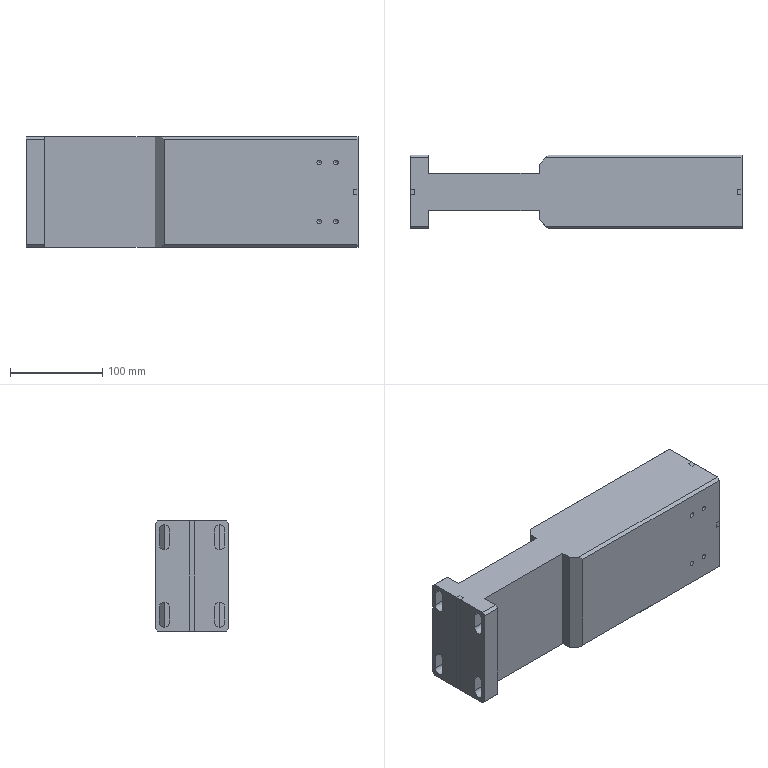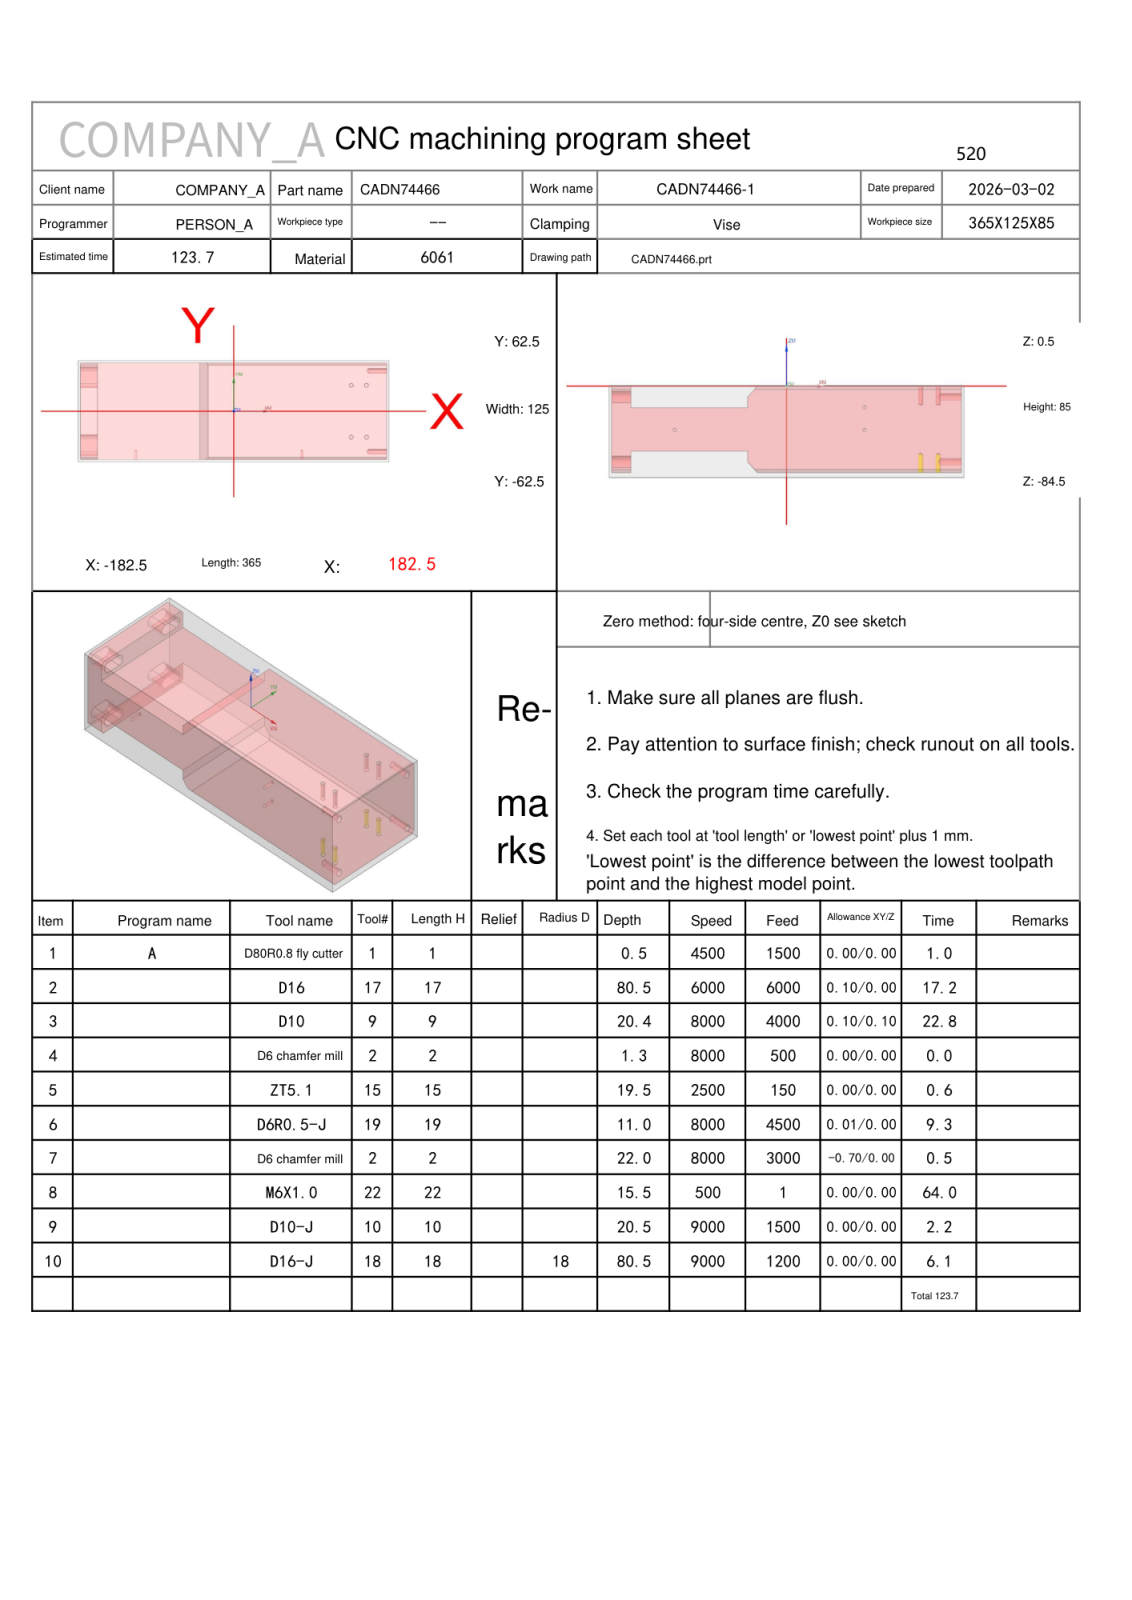NC program | NX | posted by the shop | part box 360 x 80 x 120 mm
Lines 1 to 871 of 7747:
%
O0001
(Machine time: 185.57 MIN)
(===Total Tool:9===)
(T1=D80R0.8 fly cutter D=80.  R=0.8  D-  H01 Z=0.    )
(T17=D16    D=16.  R=0.   D-  H17 Z=-80.  )
(T9=D10     D=10.  R=0.   D-  H09 Z=-19.9 )
(T2=D6 chamfer mill   D=6.   R=0.   D-  H02 Z=-21.5 )
(T15=ZT5.1  D=5.1  DR_a=118 D-  H15 Z=-19.  )
(T19=D6R0.5-J D=6.   R=0.5  D-  H19 Z=-10.5 )
(T22=M6X1.0 D=5.   DR_a=180 D-  H22 Z=-15.  )
(T10=D10-J  D=10.  R=0.   D10 H10 Z=-20.  )
(T18=D16-J  D=16.  R=0.   D18 H18 Z=-80.  )
G80 G90 G17 G49 G40
G91 G28 Z0
M01
N1 T01 M06
(D80R0.8 fly cutter  D=80. R=0.8 H=01 ce=0.00 di=0.00)
G00 G90 G54 X225. Y-50. M03 S4500
G43 H01 Z50.
M08
Z2.
G01 Z0.0 F1500.
X220.
X-220.
Y0.0
X220.
Y50.
X-220.
X-225.
Z2.
G00 Z50.
G91 G28 Z0.0
M05
M09
G91 G28 Z0.0
M01
N2 T17 M06
(D16  D=16. R=0. H=17 ce=0.10 di=0.00)
G00 G90 G54 X0.0 Y68.1 M03 S6000
G43 H17 Z50.
M08
Z.5
G01 X180. Z.358 F6000.
G02 X188.1 Y60. Z.348 I0.0 J-8.1
G01 Y-60. Z.253
G02 X180. Y-68.1 Z.243 I-8.1 J0.0
G01 X-180. Z-.04
G02 X-188.1 Y-60. Z-.05 I0.0 J8.1
G01 Y60. Z-.145
G02 X-180. Y68.1 Z-.155 I8.1 J0.0
G01 X180. Z-.439
G02 X188.1 Y60. Z-.449 I0.0 J-8.1
G01 Y-60. Z-.544
G02 X180. Y-68.1 Z-.554 I-8.1 J0.0
G01 X-180. Z-.837
G02 X-188.1 Y-60. Z-.847 I0.0 J8.1
G01 Y60. Z-.942
G02 X-180. Y68.1 Z-.952 I8.1 J0.0
G01 X180. Z-1.236
G02 X188.1 Y60. Z-1.246 I0.0 J-8.1
G01 Y-60. Z-1.341
G02 X180. Y-68.1 Z-1.351 I-8.1 J0.0
G01 X-180. Z-1.634
G02 X-188.1 Y-60. Z-1.645 I0.0 J8.1
G01 Y60. Z-1.739
G02 X-180. Y68.1 Z-1.749 I8.1 J0.0
G01 X180. Z-2.033
G02 X188.1 Y60. Z-2.043 I0.0 J-8.1
G01 Y-60. Z-2.138
G02 X180. Y-68.1 Z-2.148 I-8.1 J0.0
G01 X-180. Z-2.432
G02 X-188.1 Y-60. Z-2.442 I0.0 J8.1
G01 Y60. Z-2.536
G02 X-180. Y68.1 Z-2.546 I8.1 J0.0
G01 X180. Z-2.83
G02 X188.1 Y60. Z-2.84 I0.0 J-8.1
G01 Y-60. Z-2.935
G02 X180. Y-68.1 Z-2.945 I-8.1 J0.0
G01 X-180. Z-3.229
G02 X-188.1 Y-60. Z-3.239 I0.0 J8.1
G01 Y60. Z-3.333
G02 X-180. Y68.1 Z-3.343 I8.1 J0.0
G01 X180. Z-3.627
G02 X188.1 Y60. Z-3.637 I0.0 J-8.1
G01 Y-60. Z-3.732
G02 X180. Y-68.1 Z-3.742 I-8.1 J0.0
G01 X-180. Z-4.026
G02 X-188.1 Y-60. Z-4.036 I0.0 J8.1
G01 Y60. Z-4.13
G02 X-180. Y68.1 Z-4.14 I8.1 J0.0
G01 X180. Z-4.424
G02 X188.1 Y60. Z-4.434 I0.0 J-8.1
G01 Y-60. Z-4.529
G02 X180. Y-68.1 Z-4.539 I-8.1 J0.0
G01 X-180. Z-4.823
G02 X-188.1 Y-60. Z-4.833 I0.0 J8.1
G01 Y60. Z-4.927
G02 X-180. Y68.1 Z-4.937 I8.1 J0.0
G01 X180. Z-5.221
G02 X188.1 Y60. Z-5.231 I0.0 J-8.1
G01 Y-60. Z-5.326
G02 X180. Y-68.1 Z-5.336 I-8.1 J0.0
G01 X-180. Z-5.62
G02 X-188.1 Y-60. Z-5.63 I0.0 J8.1
G01 Y60. Z-5.724
G02 X-180. Y68.1 Z-5.734 I8.1 J0.0
G01 X180. Z-6.018
G02 X188.1 Y60. Z-6.028 I0.0 J-8.1
G01 Y-60. Z-6.123
G02 X180. Y-68.1 Z-6.133 I-8.1 J0.0
G01 X-180. Z-6.417
G02 X-188.1 Y-60. Z-6.427 I0.0 J8.1
G01 Y60. Z-6.521
G02 X-180. Y68.1 Z-6.531 I8.1 J0.0
G01 X180. Z-6.815
G02 X188.1 Y60. Z-6.825 I0.0 J-8.1
G01 Y-60. Z-6.92
G02 X180. Y-68.1 Z-6.93 I-8.1 J0.0
G01 X-180. Z-7.214
G02 X-188.1 Y-60. Z-7.224 I0.0 J8.1
G01 Y60. Z-7.318
G02 X-180. Y68.1 Z-7.328 I8.1 J0.0
G01 X180. Z-7.612
G02 X188.1 Y60. Z-7.622 I0.0 J-8.1
G01 Y-60. Z-7.717
G02 X180. Y-68.1 Z-7.727 I-8.1 J0.0
G01 X-180. Z-8.011
G02 X-188.1 Y-60. Z-8.021 I0.0 J8.1
G01 Y60. Z-8.115
G02 X-180. Y68.1 Z-8.125 I8.1 J0.0
G01 X180. Z-8.409
G02 X188.1 Y60. Z-8.419 I0.0 J-8.1
G01 Y-60. Z-8.514
G02 X180. Y-68.1 Z-8.524 I-8.1 J0.0
G01 X-180. Z-8.808
G02 X-188.1 Y-60. Z-8.818 I0.0 J8.1
G01 Y60. Z-8.912
G02 X-180. Y68.1 Z-8.922 I8.1 J0.0
G01 X180. Z-9.206
G02 X188.1 Y60. Z-9.216 I0.0 J-8.1
G01 Y-60. Z-9.311
G02 X180. Y-68.1 Z-9.321 I-8.1 J0.0
G01 X-180. Z-9.605
G02 X-188.1 Y-60. Z-9.615 I0.0 J8.1
G01 Y60. Z-9.709
G02 X-180. Y68.1 Z-9.719 I8.1 J0.0
G01 X180. Z-10.003
G02 X188.1 Y60. Z-10.013 I0.0 J-8.1
G01 Y-60. Z-10.108
G02 X180. Y-68.1 Z-10.118 I-8.1 J0.0
G01 X-180. Z-10.402
G02 X-188.1 Y-60. Z-10.412 I0.0 J8.1
G01 Y60. Z-10.506
G02 X-180. Y68.1 Z-10.516 I8.1 J0.0
G01 X180. Z-10.8
G02 X188.1 Y60. Z-10.81 I0.0 J-8.1
G01 Y-60. Z-10.905
G02 X180. Y-68.1 Z-10.915 I-8.1 J0.0
G01 X-180. Z-11.199
G02 X-188.1 Y-60. Z-11.209 I0.0 J8.1
G01 Y60. Z-11.303
G02 X-180. Y68.1 Z-11.314 I8.1 J0.0
G01 X180. Z-11.597
G02 X188.1 Y60. Z-11.607 I0.0 J-8.1
G01 Y-60. Z-11.702
G02 X180. Y-68.1 Z-11.712 I-8.1 J0.0
G01 X-180. Z-11.996
G02 X-188.1 Y-60. Z-12.006 I0.0 J8.1
G01 Y60. Z-12.101
G02 X-180. Y68.1 Z-12.111 I8.1 J0.0
G01 X180. Z-12.394
G02 X188.1 Y60. Z-12.404 I0.0 J-8.1
G01 Y-60. Z-12.499
G02 X180. Y-68.1 Z-12.509 I-8.1 J0.0
G01 X-180. Z-12.793
G02 X-188.1 Y-60. Z-12.803 I0.0 J8.1
G01 Y60. Z-12.898
G02 X-180. Y68.1 Z-12.908 I8.1 J0.0
G01 X180. Z-13.191
G02 X188.1 Y60. Z-13.201 I0.0 J-8.1
G01 Y-60. Z-13.296
G02 X180. Y-68.1 Z-13.306 I-8.1 J0.0
G01 X-180. Z-13.59
G02 X-188.1 Y-60. Z-13.6 I0.0 J8.1
G01 Y60. Z-13.695
G02 X-180. Y68.1 Z-13.705 I8.1 J0.0
G01 X180. Z-13.988
G02 X188.1 Y60. Z-13.998 I0.0 J-8.1
G01 Y-60. Z-14.093
G02 X180. Y-68.1 Z-14.103 I-8.1 J0.0
G01 X-180. Z-14.387
G02 X-188.1 Y-60. Z-14.397 I0.0 J8.1
G01 Y60. Z-14.492
G02 X-180. Y68.1 Z-14.502 I8.1 J0.0
G01 X180. Z-14.785
G02 X188.1 Y60. Z-14.796 I0.0 J-8.1
G01 Y-60. Z-14.89
G02 X180. Y-68.1 Z-14.9 I-8.1 J0.0
G01 X-180. Z-15.184
G02 X-188.1 Y-60. Z-15.194 I0.0 J8.1
G01 Y60. Z-15.289
G02 X-180. Y68.1 Z-15.299 I8.1 J0.0
G01 X180. Z-15.583
G02 X188.1 Y60. Z-15.593 I0.0 J-8.1
G01 Y-60. Z-15.687
G02 X180. Y-68.1 Z-15.697 I-8.1 J0.0
G01 X-180. Z-15.981
G02 X-188.1 Y-60. Z-15.991 I0.0 J8.1
G01 Y60. Z-16.086
G02 X-180. Y68.1 Z-16.096 I8.1 J0.0
G01 X180. Z-16.38
G02 X188.1 Y60. Z-16.39 I0.0 J-8.1
G01 Y-60. Z-16.484
G02 X180. Y-68.1 Z-16.494 I-8.1 J0.0
G01 X-180. Z-16.778
G02 X-188.1 Y-60. Z-16.788 I0.0 J8.1
G01 Y60. Z-16.883
G02 X-180. Y68.1 Z-16.893 I8.1 J0.0
G01 X180. Z-17.177
G02 X188.1 Y60. Z-17.187 I0.0 J-8.1
G01 Y-60. Z-17.281
G02 X180. Y-68.1 Z-17.291 I-8.1 J0.0
G01 X-180. Z-17.575
G02 X-188.1 Y-60. Z-17.585 I0.0 J8.1
G01 Y60. Z-17.68
G02 X-180. Y68.1 Z-17.69 I8.1 J0.0
G01 X180. Z-17.974
G02 X188.1 Y60. Z-17.984 I0.0 J-8.1
G01 Y-60. Z-18.078
G02 X180. Y-68.1 Z-18.088 I-8.1 J0.0
G01 X-180. Z-18.372
G02 X-188.1 Y-60. Z-18.382 I0.0 J8.1
G01 Y60. Z-18.477
G02 X-180. Y68.1 Z-18.487 I8.1 J0.0
G01 X180. Z-18.771
G02 X188.1 Y60. Z-18.781 I0.0 J-8.1
G01 Y-60. Z-18.875
G02 X180. Y-68.1 Z-18.885 I-8.1 J0.0
G01 X-180. Z-19.169
G02 X-188.1 Y-60. Z-19.179 I0.0 J8.1
G01 Y60. Z-19.274
G02 X-180. Y68.1 Z-19.284 I8.1 J0.0
G01 X180. Z-19.568
G02 X188.1 Y60. Z-19.578 I0.0 J-8.1
G01 Y-60. Z-19.672
G02 X180. Y-68.1 Z-19.682 I-8.1 J0.0
G01 X-180. Z-19.966
G02 X-188.1 Y-60. Z-19.976 I0.0 J8.1
G01 Y60. Z-20.071
G02 X-180. Y68.1 Z-20.081 I8.1 J0.0
G01 X180. Z-20.365
G02 X188.1 Y60. Z-20.375 I0.0 J-8.1
G01 Y-60. Z-20.469
G02 X180. Y-68.1 Z-20.479 I-8.1 J0.0
G01 X-180. Z-20.763
G02 X-188.1 Y-60. Z-20.773 I0.0 J8.1
G01 Y60. Z-20.868
G02 X-180. Y68.1 Z-20.878 I8.1 J0.0
G01 X180. Z-21.162
G02 X188.1 Y60. Z-21.172 I0.0 J-8.1
G01 Y-60. Z-21.266
G02 X180. Y-68.1 Z-21.276 I-8.1 J0.0
G01 X-180. Z-21.56
G02 X-188.1 Y-60. Z-21.57 I0.0 J8.1
G01 Y60. Z-21.665
G02 X-180. Y68.1 Z-21.675 I8.1 J0.0
G01 X180. Z-21.959
G02 X188.1 Y60. Z-21.969 I0.0 J-8.1
G01 Y-60. Z-22.063
G02 X180. Y-68.1 Z-22.073 I-8.1 J0.0
G01 X-180. Z-22.357
G02 X-188.1 Y-60. Z-22.367 I0.0 J8.1
G01 Y60. Z-22.462
G02 X-180. Y68.1 Z-22.472 I8.1 J0.0
G01 X180. Z-22.756
G02 X188.1 Y60. Z-22.766 I0.0 J-8.1
G01 Y-60. Z-22.86
G02 X180. Y-68.1 Z-22.87 I-8.1 J0.0
G01 X-180. Z-23.154
G02 X-188.1 Y-60. Z-23.164 I0.0 J8.1
G01 Y60. Z-23.259
G02 X-180. Y68.1 Z-23.269 I8.1 J0.0
G01 X180. Z-23.553
G02 X188.1 Y60. Z-23.563 I0.0 J-8.1
G01 Y-60. Z-23.657
G02 X180. Y-68.1 Z-23.667 I-8.1 J0.0
G01 X-180. Z-23.951
G02 X-188.1 Y-60. Z-23.961 I0.0 J8.1
G01 Y60. Z-24.056
G02 X-180. Y68.1 Z-24.066 I8.1 J0.0
G01 X180. Z-24.35
G02 X188.1 Y60. Z-24.36 I0.0 J-8.1
G01 Y-60. Z-24.454
G02 X180. Y-68.1 Z-24.465 I-8.1 J0.0
G01 X-180. Z-24.748
G02 X-188.1 Y-60. Z-24.758 I0.0 J8.1
G01 Y60. Z-24.853
G02 X-180. Y68.1 Z-24.863 I8.1 J0.0
G01 X180. Z-25.147
G02 X188.1 Y60. Z-25.157 I0.0 J-8.1
G01 Y-60. Z-25.252
G02 X180. Y-68.1 Z-25.262 I-8.1 J0.0
G01 X-180. Z-25.545
G02 X-188.1 Y-60. Z-25.555 I0.0 J8.1
G01 Y60. Z-25.65
G02 X-180. Y68.1 Z-25.66 I8.1 J0.0
G01 X180. Z-25.944
G02 X188.1 Y60. Z-25.954 I0.0 J-8.1
G01 Y-60. Z-26.049
G02 X180. Y-68.1 Z-26.059 I-8.1 J0.0
G01 X-180. Z-26.342
G02 X-188.1 Y-60. Z-26.352 I0.0 J8.1
G01 Y60. Z-26.447
G02 X-180. Y68.1 Z-26.457 I8.1 J0.0
G01 X180. Z-26.741
G02 X188.1 Y60. Z-26.751 I0.0 J-8.1
G01 Y-60. Z-26.846
G02 X180. Y-68.1 Z-26.856 I-8.1 J0.0
G01 X-180. Z-27.139
G02 X-188.1 Y-60. Z-27.149 I0.0 J8.1
G01 Y60. Z-27.244
G02 X-180. Y68.1 Z-27.254 I8.1 J0.0
G01 X180. Z-27.538
G02 X188.1 Y60. Z-27.548 I0.0 J-8.1
G01 Y-60. Z-27.643
G02 X180. Y-68.1 Z-27.653 I-8.1 J0.0
G01 X-180. Z-27.936
G02 X-188.1 Y-60. Z-27.947 I0.0 J8.1
G01 Y60. Z-28.041
G02 X-180. Y68.1 Z-28.051 I8.1 J0.0
G01 X180. Z-28.335
G02 X188.1 Y60. Z-28.345 I0.0 J-8.1
G01 Y-60. Z-28.44
G02 X180. Y-68.1 Z-28.45 I-8.1 J0.0
G01 X-180. Z-28.734
G02 X-188.1 Y-60. Z-28.744 I0.0 J8.1
G01 Y60. Z-28.838
G02 X-180. Y68.1 Z-28.848 I8.1 J0.0
G01 X180. Z-29.132
G02 X188.1 Y60. Z-29.142 I0.0 J-8.1
G01 Y-60. Z-29.237
G02 X180. Y-68.1 Z-29.247 I-8.1 J0.0
G01 X-180. Z-29.531
G02 X-188.1 Y-60. Z-29.541 I0.0 J8.1
G01 Y60. Z-29.635
G02 X-180. Y68.1 Z-29.645 I8.1 J0.0
G01 X180. Z-29.929
G02 X188.1 Y60. Z-29.939 I0.0 J-8.1
G01 Y-60. Z-30.034
G02 X180. Y-68.1 Z-30.044 I-8.1 J0.0
G01 X-180. Z-30.328
G02 X-188.1 Y-60. Z-30.338 I0.0 J8.1
G01 Y60. Z-30.432
G02 X-180. Y68.1 Z-30.442 I8.1 J0.0
G01 X180. Z-30.726
G02 X188.1 Y60. Z-30.736 I0.0 J-8.1
G01 Y-60. Z-30.831
G02 X180. Y-68.1 Z-30.841 I-8.1 J0.0
G01 X-180. Z-31.125
G02 X-188.1 Y-60. Z-31.135 I0.0 J8.1
G01 Y60. Z-31.229
G02 X-180. Y68.1 Z-31.239 I8.1 J0.0
G01 X180. Z-31.523
G02 X188.1 Y60. Z-31.533 I0.0 J-8.1
G01 Y-60. Z-31.628
G02 X180. Y-68.1 Z-31.638 I-8.1 J0.0
G01 X-180. Z-31.922
G02 X-188.1 Y-60. Z-31.932 I0.0 J8.1
G01 Y60. Z-32.026
G02 X-180. Y68.1 Z-32.036 I8.1 J0.0
G01 X180. Z-32.32
G02 X188.1 Y60. Z-32.33 I0.0 J-8.1
G01 Y-60. Z-32.425
G02 X180. Y-68.1 Z-32.435 I-8.1 J0.0
G01 X-180. Z-32.719
G02 X-188.1 Y-60. Z-32.729 I0.0 J8.1
G01 Y60. Z-32.823
G02 X-180. Y68.1 Z-32.833 I8.1 J0.0
G01 X180. Z-33.117
G02 X188.1 Y60. Z-33.127 I0.0 J-8.1
G01 Y-60. Z-33.222
G02 X180. Y-68.1 Z-33.232 I-8.1 J0.0
G01 X-180. Z-33.516
G02 X-188.1 Y-60. Z-33.526 I0.0 J8.1
G01 Y60. Z-33.62
G02 X-180. Y68.1 Z-33.63 I8.1 J0.0
G01 X180. Z-33.914
G02 X188.1 Y60. Z-33.924 I0.0 J-8.1
G01 Y-60. Z-34.019
G02 X180. Y-68.1 Z-34.029 I-8.1 J0.0
G01 X-180. Z-34.313
G02 X-188.1 Y-60. Z-34.323 I0.0 J8.1
G01 Y60. Z-34.417
G02 X-180. Y68.1 Z-34.427 I8.1 J0.0
G01 X180. Z-34.711
G02 X188.1 Y60. Z-34.721 I0.0 J-8.1
G01 Y-60. Z-34.816
G02 X180. Y-68.1 Z-34.826 I-8.1 J0.0
G01 X-180. Z-35.11
G02 X-188.1 Y-60. Z-35.12 I0.0 J8.1
G01 Y60. Z-35.214
G02 X-180. Y68.1 Z-35.224 I8.1 J0.0
G01 X180. Z-35.508
G02 X188.1 Y60. Z-35.518 I0.0 J-8.1
G01 Y-60. Z-35.613
G02 X180. Y-68.1 Z-35.623 I-8.1 J0.0
G01 X-180. Z-35.907
G02 X-188.1 Y-60. Z-35.917 I0.0 J8.1
G01 Y60. Z-36.011
G02 X-180. Y68.1 Z-36.021 I8.1 J0.0
G01 X180. Z-36.305
G02 X188.1 Y60. Z-36.315 I0.0 J-8.1
G01 Y-60. Z-36.41
G02 X180. Y-68.1 Z-36.42 I-8.1 J0.0
G01 X-180. Z-36.704
G02 X-188.1 Y-60. Z-36.714 I0.0 J8.1
G01 Y60. Z-36.808
G02 X-180. Y68.1 Z-36.818 I8.1 J0.0
G01 X180. Z-37.102
G02 X188.1 Y60. Z-37.112 I0.0 J-8.1
G01 Y-60. Z-37.207
G02 X180. Y-68.1 Z-37.217 I-8.1 J0.0
G01 X-180. Z-37.501
G02 X-188.1 Y-60. Z-37.511 I0.0 J8.1
G01 Y60. Z-37.605
G02 X-180. Y68.1 Z-37.616 I8.1 J0.0
G01 X180. Z-37.899
G02 X188.1 Y60. Z-37.909 I0.0 J-8.1
G01 Y-60. Z-38.004
G02 X180. Y-68.1 Z-38.014 I-8.1 J0.0
G01 X-180. Z-38.298
G02 X-188.1 Y-60. Z-38.308 I0.0 J8.1
G01 Y60. Z-38.403
G02 X-180. Y68.1 Z-38.413 I8.1 J0.0
G01 X180. Z-38.696
G02 X188.1 Y60. Z-38.706 I0.0 J-8.1
G01 Y-60. Z-38.801
G02 X180. Y-68.1 Z-38.811 I-8.1 J0.0
G01 X-180. Z-39.095
G02 X-188.1 Y-60. Z-39.105 I0.0 J8.1
G01 Y60. Z-39.2
G02 X-180. Y68.1 Z-39.21 I8.1 J0.0
G01 X180. Z-39.493
G02 X188.1 Y60. Z-39.503 I0.0 J-8.1
G01 Y-60. Z-39.598
G02 X180. Y-68.1 Z-39.608 I-8.1 J0.0
G01 X-180. Z-39.892
G02 X-188.1 Y-60. Z-39.902 I0.0 J8.1
G01 Y60. Z-39.997
G02 X-180. Y68.1 Z-40.007 I8.1 J0.0
G01 X180. Z-40.29
G02 X188.1 Y60. Z-40.3 I0.0 J-8.1
G01 Y-60. Z-40.395
G02 X180. Y-68.1 Z-40.405 I-8.1 J0.0
G01 X-180. Z-40.689
G02 X-188.1 Y-60. Z-40.699 I0.0 J8.1
G01 Y60. Z-40.794
G02 X-180. Y68.1 Z-40.804 I8.1 J0.0
G01 X180. Z-41.087
G02 X188.1 Y60. Z-41.097 I0.0 J-8.1
G01 Y-60. Z-41.192
G02 X180. Y-68.1 Z-41.202 I-8.1 J0.0
G01 X-180. Z-41.486
G02 X-188.1 Y-60. Z-41.496 I0.0 J8.1
G01 Y60. Z-41.591
G02 X-180. Y68.1 Z-41.601 I8.1 J0.0
G01 X180. Z-41.884
G02 X188.1 Y60. Z-41.895 I0.0 J-8.1
G01 Y-60. Z-41.989
G02 X180. Y-68.1 Z-41.999 I-8.1 J0.0
G01 X-180. Z-42.283
G02 X-188.1 Y-60. Z-42.293 I0.0 J8.1
G01 Y60. Z-42.388
G02 X-180. Y68.1 Z-42.398 I8.1 J0.0
G01 X180. Z-42.682
G02 X188.1 Y60. Z-42.692 I0.0 J-8.1
G01 Y-60. Z-42.786
G02 X180. Y-68.1 Z-42.796 I-8.1 J0.0
G01 X-180. Z-43.08
G02 X-188.1 Y-60. Z-43.09 I0.0 J8.1
G01 Y60. Z-43.185
G02 X-180. Y68.1 Z-43.195 I8.1 J0.0
G01 X180. Z-43.479
G02 X188.1 Y60. Z-43.489 I0.0 J-8.1
G01 Y-60. Z-43.583
G02 X180. Y-68.1 Z-43.593 I-8.1 J0.0
G01 X-180. Z-43.877
G02 X-188.1 Y-60. Z-43.887 I0.0 J8.1
G01 Y60. Z-43.982
G02 X-180. Y68.1 Z-43.992 I8.1 J0.0
G01 X180. Z-44.276
G02 X188.1 Y60. Z-44.286 I0.0 J-8.1
G01 Y-60. Z-44.38
G02 X180. Y-68.1 Z-44.39 I-8.1 J0.0
G01 X-180. Z-44.674
G02 X-188.1 Y-60. Z-44.684 I0.0 J8.1
G01 Y60. Z-44.779
G02 X-180. Y68.1 Z-44.789 I8.1 J0.0
G01 X180. Z-45.073
G02 X188.1 Y60. Z-45.083 I0.0 J-8.1
G01 Y-60. Z-45.177
G02 X180. Y-68.1 Z-45.187 I-8.1 J0.0
G01 X-180. Z-45.471
G02 X-188.1 Y-60. Z-45.481 I0.0 J8.1
G01 Y60. Z-45.576
G02 X-180. Y68.1 Z-45.586 I8.1 J0.0
G01 X180. Z-45.87
G02 X188.1 Y60. Z-45.88 I0.0 J-8.1
G01 Y-60. Z-45.974
G02 X180. Y-68.1 Z-45.984 I-8.1 J0.0
G01 X-180. Z-46.268
G02 X-188.1 Y-60. Z-46.278 I0.0 J8.1
G01 Y60. Z-46.373
G02 X-180. Y68.1 Z-46.383 I8.1 J0.0
G01 X180. Z-46.667
G02 X188.1 Y60. Z-46.677 I0.0 J-8.1
G01 Y-60. Z-46.771
G02 X180. Y-68.1 Z-46.781 I-8.1 J0.0
G01 X-180. Z-47.065
G02 X-188.1 Y-60. Z-47.075 I0.0 J8.1
G01 Y60. Z-47.17
G02 X-180. Y68.1 Z-47.18 I8.1 J0.0
G01 X180. Z-47.464
G02 X188.1 Y60. Z-47.474 I0.0 J-8.1
G01 Y-60. Z-47.568
G02 X180. Y-68.1 Z-47.578 I-8.1 J0.0
G01 X-180. Z-47.862
G02 X-188.1 Y-60. Z-47.872 I0.0 J8.1
G01 Y60. Z-47.967
G02 X-180. Y68.1 Z-47.977 I8.1 J0.0
G01 X180. Z-48.261
G02 X188.1 Y60. Z-48.271 I0.0 J-8.1
G01 Y-60. Z-48.365
G02 X180. Y-68.1 Z-48.375 I-8.1 J0.0
G01 X-180. Z-48.659
G02 X-188.1 Y-60. Z-48.669 I0.0 J8.1
G01 Y60. Z-48.764
G02 X-180. Y68.1 Z-48.774 I8.1 J0.0
G01 X180. Z-49.058
G02 X188.1 Y60. Z-49.068 I0.0 J-8.1
G01 Y-60. Z-49.162
G02 X180. Y-68.1 Z-49.172 I-8.1 J0.0
G01 X-180. Z-49.456
G02 X-188.1 Y-60. Z-49.466 I0.0 J8.1
G01 Y60. Z-49.561
G02 X-180. Y68.1 Z-49.571 I8.1 J0.0
G01 X180. Z-49.855
G02 X188.1 Y60. Z-49.865 I0.0 J-8.1
G01 Y-60. Z-49.959
G02 X180. Y-68.1 Z-49.969 I-8.1 J0.0
G01 X-180. Z-50.253
G02 X-188.1 Y-60. Z-50.263 I0.0 J8.1
G01 Y60. Z-50.358
G02 X-180. Y68.1 Z-50.368 I8.1 J0.0
G01 X180. Z-50.652
G02 X188.1 Y60. Z-50.662 I0.0 J-8.1
G01 Y-60. Z-50.756
G02 X180. Y-68.1 Z-50.766 I-8.1 J0.0
G01 X-180. Z-51.05
G02 X-188.1 Y-60. Z-51.06 I0.0 J8.1
G01 Y60. Z-51.155
G02 X-180. Y68.1 Z-51.165 I8.1 J0.0
G01 X180. Z-51.449
G02 X188.1 Y60. Z-51.459 I0.0 J-8.1
G01 Y-60. Z-51.553
G02 X180. Y-68.1 Z-51.564 I-8.1 J0.0
G01 X-180. Z-51.847
G02 X-188.1 Y-60. Z-51.857 I0.0 J8.1
G01 Y60. Z-51.952
G02 X-180. Y68.1 Z-51.962 I8.1 J0.0
G01 X180. Z-52.246
G02 X188.1 Y60. Z-52.256 I0.0 J-8.1
G01 Y-60. Z-52.351
G02 X180. Y-68.1 Z-52.361 I-8.1 J0.0
G01 X-180. Z-52.644
G02 X-188.1 Y-60. Z-52.654 I0.0 J8.1
G01 Y60. Z-52.749
G02 X-180. Y68.1 Z-52.759 I8.1 J0.0
G01 X180. Z-53.043
G02 X188.1 Y60. Z-53.053 I0.0 J-8.1
G01 Y-60. Z-53.148
G02 X180. Y-68.1 Z-53.158 I-8.1 J0.0
G01 X-180. Z-53.441
G02 X-188.1 Y-60. Z-53.451 I0.0 J8.1
G01 Y60. Z-53.546
G02 X-180. Y68.1 Z-53.556 I8.1 J0.0
G01 X180. Z-53.84
G02 X188.1 Y60. Z-53.85 I0.0 J-8.1
G01 Y-60. Z-53.945
G02 X180. Y-68.1 Z-53.955 I-8.1 J0.0
G01 X-180. Z-54.238
G02 X-188.1 Y-60. Z-54.248 I0.0 J8.1
G01 Y60. Z-54.343
G02 X-180. Y68.1 Z-54.353 I8.1 J0.0
G01 X180. Z-54.637
G02 X188.1 Y60. Z-54.647 I0.0 J-8.1
G01 Y-60. Z-54.742
G02 X180. Y-68.1 Z-54.752 I-8.1 J0.0
G01 X-180. Z-55.035
G02 X-188.1 Y-60. Z-55.046 I0.0 J8.1
G01 Y60. Z-55.14
G02 X-180. Y68.1 Z-55.15 I8.1 J0.0
G01 X180. Z-55.434
G02 X188.1 Y60. Z-55.444 I0.0 J-8.1
G01 Y-60. Z-55.539
G02 X180. Y-68.1 Z-55.549 I-8.1 J0.0
G01 X-180. Z-55.833
G02 X-188.1 Y-60. Z-55.843 I0.0 J8.1
G01 Y60. Z-55.937
G02 X-180. Y68.1 Z-55.947 I8.1 J0.0
G01 X180. Z-56.231
G02 X188.1 Y60. Z-56.241 I0.0 J-8.1
G01 Y-60. Z-56.336
G02 X180. Y-68.1 Z-56.346 I-8.1 J0.0
G01 X-180. Z-56.63
G02 X-188.1 Y-60. Z-56.64 I0.0 J8.1
G01 Y60. Z-56.734
G02 X-180. Y68.1 Z-56.744 I8.1 J0.0
G01 X180. Z-57.028
G02 X188.1 Y60. Z-57.038 I0.0 J-8.1
G01 Y-60. Z-57.133
G02 X180. Y-68.1 Z-57.143 I-8.1 J0.0
G01 X-180. Z-57.427
G02 X-188.1 Y-60. Z-57.437 I0.0 J8.1
G01 Y60. Z-57.531
G02 X-180. Y68.1 Z-57.541 I8.1 J0.0
G01 X180. Z-57.825
G02 X188.1 Y60. Z-57.835 I0.0 J-8.1
G01 Y-60. Z-57.93
G02 X180. Y-68.1 Z-57.94 I-8.1 J0.0
G01 X-180. Z-58.224
G02 X-188.1 Y-60. Z-58.234 I0.0 J8.1
G01 Y60. Z-58.328
G02 X-180. Y68.1 Z-58.338 I8.1 J0.0
G01 X180. Z-58.622
G02 X188.1 Y60. Z-58.632 I0.0 J-8.1
G01 Y-60. Z-58.727
G02 X180. Y-68.1 Z-58.737 I-8.1 J0.0
G01 X-180. Z-59.021
G02 X-188.1 Y-60. Z-59.031 I0.0 J8.1
G01 Y60. Z-59.125
G02 X-180. Y68.1 Z-59.135 I8.1 J0.0
G01 X180. Z-59.419
G02 X188.1 Y60. Z-59.429 I0.0 J-8.1
G01 Y-60. Z-59.524
G02 X180. Y-68.1 Z-59.534 I-8.1 J0.0
G01 X-180. Z-59.818
G02 X-188.1 Y-60. Z-59.828 I0.0 J8.1
G01 Y60. Z-59.922
G02 X-180. Y68.1 Z-59.932 I8.1 J0.0
G01 X180. Z-60.216
G02 X188.1 Y60. Z-60.226 I0.0 J-8.1
G01 Y-60. Z-60.321
G02 X180. Y-68.1 Z-60.331 I-8.1 J0.0
G01 X-180. Z-60.615
G02 X-188.1 Y-60. Z-60.625 I0.0 J8.1
G01 Y60. Z-60.719
G02 X-180. Y68.1 Z-60.729 I8.1 J0.0
G01 X180. Z-61.013
G02 X188.1 Y60. Z-61.023 I0.0 J-8.1
G01 Y-60. Z-61.118
G02 X180. Y-68.1 Z-61.128 I-8.1 J0.0
G01 X-180. Z-61.412
G02 X-188.1 Y-60. Z-61.422 I0.0 J8.1
G01 Y60. Z-61.516
G02 X-180. Y68.1 Z-61.526 I8.1 J0.0
G01 X180. Z-61.81
G02 X188.1 Y60. Z-61.82 I0.0 J-8.1
G01 Y-60. Z-61.915
G02 X180. Y-68.1 Z-61.925 I-8.1 J0.0
G01 X-180. Z-62.209
G02 X-188.1 Y-60. Z-62.219 I0.0 J8.1
G01 Y60. Z-62.313
G02 X-180. Y68.1 Z-62.323 I8.1 J0.0
G01 X180. Z-62.607
G02 X188.1 Y60. Z-62.617 I0.0 J-8.1
G01 Y-60. Z-62.712
G02 X180. Y-68.1 Z-62.722 I-8.1 J0.0
G01 X-180. Z-63.006
G02 X-188.1 Y-60. Z-63.016 I0.0 J8.1
G01 Y60. Z-63.11
G02 X-180. Y68.1 Z-63.12 I8.1 J0.0
G01 X180. Z-63.404
G02 X188.1 Y60. Z-63.414 I0.0 J-8.1
G01 Y-60. Z-63.509
G02 X180. Y-68.1 Z-63.519 I-8.1 J0.0
G01 X-180. Z-63.803
G02 X-188.1 Y-60. Z-63.813 I0.0 J8.1
G01 Y60. Z-63.907
G02 X-180. Y68.1 Z-63.917 I8.1 J0.0
G01 X180. Z-64.201
G02 X188.1 Y60. Z-64.211 I0.0 J-8.1
G01 Y-60. Z-64.306
G02 X180. Y-68.1 Z-64.316 I-8.1 J0.0
G01 X-180. Z-64.6
G02 X-188.1 Y-60. Z-64.61 I0.0 J8.1
G01 Y60. Z-64.704
G02 X-180. Y68.1 Z-64.715 I8.1 J0.0
G01 X180. Z-64.998
G02 X188.1 Y60. Z-65.008 I0.0 J-8.1
G01 Y-60. Z-65.103
G02 X180. Y-68.1 Z-65.113 I-8.1 J0.0
G01 X-180. Z-65.397
G02 X-188.1 Y-60. Z-65.407 I0.0 J8.1
G01 Y60. Z-65.502
G02 X-180. Y68.1 Z-65.512 I8.1 J0.0
G01 X180. Z-65.795
G02 X188.1 Y60. Z-65.805 I0.0 J-8.1
G01 Y-60. Z-65.9
G02 X180. Y-68.1 Z-65.91 I-8.1 J0.0
G01 X-180. Z-66.194
G02 X-188.1 Y-60. Z-66.204 I0.0 J8.1
G01 Y60. Z-66.299
G02 X-180. Y68.1 Z-66.309 I8.1 J0.0
G01 X180. Z-66.592
G02 X188.1 Y60. Z-66.602 I0.0 J-8.1
G01 Y-60. Z-66.697
G02 X180. Y-68.1 Z-66.707 I-8.1 J0.0
G01 X-180. Z-66.991
G02 X-188.1 Y-60. Z-67.001 I0.0 J8.1
G01 Y60. Z-67.096
G02 X-180. Y68.1 Z-67.106 I8.1 J0.0
G01 X180. Z-67.389
G02 X188.1 Y60. Z-67.399 I0.0 J-8.1
G01 Y-60. Z-67.494
G02 X180. Y-68.1 Z-67.504 I-8.1 J0.0
G01 X-180. Z-67.788
G02 X-188.1 Y-60. Z-67.798 I0.0 J8.1
G01 Y60. Z-67.893
G02 X-180. Y68.1 Z-67.903 I8.1 J0.0
G01 X180. Z-68.186
G02 X188.1 Y60. Z-68.197 I0.0 J-8.1
G01 Y-60. Z-68.291
G02 X180. Y-68.1 Z-68.301 I-8.1 J0.0
G01 X-180. Z-68.585
G02 X-188.1 Y-60. Z-68.595 I0.0 J8.1
G01 Y60. Z-68.69
G02 X-180. Y68.1 Z-68.7 I8.1 J0.0
G01 X180. Z-68.984
G02 X188.1 Y60. Z-68.994 I0.0 J-8.1
G01 Y-60. Z-69.088
G02 X180. Y-68.1 Z-69.098 I-8.1 J0.0
G01 X-180. Z-69.382
G02 X-188.1 Y-60. Z-69.392 I0.0 J8.1
G01 Y60. Z-69.487
G02 X-180. Y68.1 Z-69.497 I8.1 J0.0
G01 X180. Z-69.781
G02 X188.1 Y60. Z-69.791 I0.0 J-8.1
G01 Y-60. Z-69.885
G02 X180. Y-68.1 Z-69.895 I-8.1 J0.0
G01 X-180. Z-70.179
G02 X-188.1 Y-60. Z-70.189 I0.0 J8.1
G01 Y60. Z-70.284
G02 X-180. Y68.1 Z-70.294 I8.1 J0.0
G01 X180. Z-70.578
G02 X188.1 Y60. Z-70.588 I0.0 J-8.1
G01 Y-60. Z-70.682
G02 X180. Y-68.1 Z-70.692 I-8.1 J0.0
G01 X-180. Z-70.976
G02 X-188.1 Y-60. Z-70.986 I0.0 J8.1
G01 Y60. Z-71.081
G02 X-180. Y68.1 Z-71.091 I8.1 J0.0
G01 X180. Z-71.375
G02 X188.1 Y60. Z-71.385 I0.0 J-8.1
G01 Y-60. Z-71.479
G02 X180. Y-68.1 Z-71.489 I-8.1 J0.0
G01 X-180. Z-71.773
G02 X-188.1 Y-60. Z-71.783 I0.0 J8.1
G01 Y60. Z-71.878
G02 X-180. Y68.1 Z-71.888 I8.1 J0.0
G01 X180. Z-72.172
G02 X188.1 Y60. Z-72.182 I0.0 J-8.1
G01 Y-60. Z-72.276
G02 X180. Y-68.1 Z-72.286 I-8.1 J0.0
G01 X-180. Z-72.57
G02 X-188.1 Y-60. Z-72.58 I0.0 J8.1
G01 Y60. Z-72.675
G02 X-180. Y68.1 Z-72.685 I8.1 J0.0
G01 X180. Z-72.969
G02 X188.1 Y60. Z-72.979 I0.0 J-8.1
G01 Y-60. Z-73.073
G02 X180. Y-68.1 Z-73.083 I-8.1 J0.0
G01 X-180. Z-73.367
G02 X-188.1 Y-60. Z-73.377 I0.0 J8.1
G01 Y60. Z-73.472
G02 X-180. Y68.1 Z-73.482 I8.1 J0.0
G01 X180. Z-73.766
G02 X188.1 Y60. Z-73.776 I0.0 J-8.1
G01 Y-60. Z-73.87
G02 X180. Y-68.1 Z-73.88 I-8.1 J0.0
G01 X-180. Z-74.164
G02 X-188.1 Y-60. Z-74.174 I0.0 J8.1
G01 Y60. Z-74.269
G02 X-180. Y68.1 Z-74.279 I8.1 J0.0
G01 X180. Z-74.563
G02 X188.1 Y60. Z-74.573 I0.0 J-8.1
G01 Y-60. Z-74.667
G02 X180. Y-68.1 Z-74.677 I-8.1 J0.0
G01 X-180. Z-74.961
G02 X-188.1 Y-60. Z-74.971 I0.0 J8.1
G01 Y60. Z-75.066
G02 X-180. Y68.1 Z-75.076 I8.1 J0.0
G01 X180. Z-75.36
G02 X188.1 Y60. Z-75.37 I0.0 J-8.1
G01 Y-60. Z-75.464
G02 X180. Y-68.1 Z-75.474 I-8.1 J0.0
G01 X-180. Z-75.758
G02 X-188.1 Y-60. Z-75.768 I0.0 J8.1
G01 Y60. Z-75.863
G02 X-180. Y68.1 Z-75.873 I8.1 J0.0
G01 X180. Z-76.157
G02 X188.1 Y60. Z-76.167 I0.0 J-8.1
G01 Y-60. Z-76.261
G02 X180. Y-68.1 Z-76.271 I-8.1 J0.0
G01 X-180. Z-76.555
G02 X-188.1 Y-60. Z-76.565 I0.0 J8.1
G01 Y60. Z-76.66
G02 X-180. Y68.1 Z-76.67 I8.1 J0.0
G01 X180. Z-76.954
G02 X188.1 Y60. Z-76.964 I0.0 J-8.1
G01 Y-60. Z-77.058
G02 X180. Y-68.1 Z-77.068 I-8.1 J0.0
G01 X-180. Z-77.352
G02 X-188.1 Y-60. Z-77.362 I0.0 J8.1
G01 Y60. Z-77.457
G02 X-180. Y68.1 Z-77.467 I8.1 J0.0
G01 X180. Z-77.751
G02 X188.1 Y60. Z-77.761 I0.0 J-8.1
G01 Y-60. Z-77.855
G02 X180. Y-68.1 Z-77.866 I-8.1 J0.0
G01 X-180. Z-78.149
G02 X-188.1 Y-60. Z-78.159 I0.0 J8.1
G01 Y60. Z-78.254
G02 X-180. Y68.1 Z-78.264 I8.1 J0.0
G01 X180. Z-78.548
G02 X188.1 Y60. Z-78.558 I0.0 J-8.1
G01 Y-60. Z-78.653
G02 X180. Y-68.1 Z-78.663 I-8.1 J0.0
G01 X-180. Z-78.946
G02 X-188.1 Y-60. Z-78.956 I0.0 J8.1
G01 Y60. Z-79.051
G02 X-180. Y68.1 Z-79.061 I8.1 J0.0
G01 X180. Z-79.345
G02 X188.1 Y60. Z-79.355 I0.0 J-8.1
G01 Y-60. Z-79.45
G02 X180. Y-68.1 Z-79.46 I-8.1 J0.0
G01 X-180. Z-79.743
G02 X-188.1 Y-60. Z-79.753 I0.0 J8.1
G01 Y60. Z-79.848
G02 X-180. Y68.1 Z-79.858 I8.1 J0.0
G01 X0.0 Z-80.
X180.
G02 X188.1 Y60. I0.0 J-8.1
G01 Y-60.
G02 X180. Y-68.1 I-8.1 J0.0
G01 X-180.
G02 X-188.1 Y-60. I0.0 J8.1
G01 Y60.
G02 X-180. Y68.1 I8.1 J0.0
G01 X0.0
X.5
Z-79.
G00 Z50.
G91 G28 Z0.0
M05
M09
G91 G28 Z0.0
M01